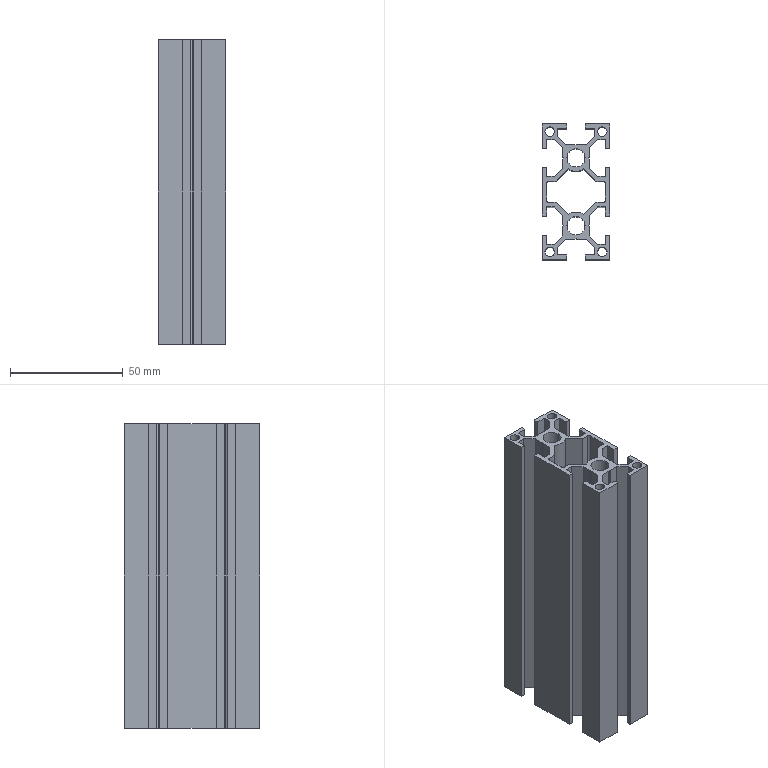Part | STEP file | BPSP-03-003 Aluminium Profile01_Default<As Machined> | 1 solid | 116 faces | box 30 x 60 x 135 mm | volume 76001 mm3 | plane 94 | cylinder 22 | commonest cylinder face diameters 4.2 x8 0.6 x4 2 x4 8 x4 12 x2